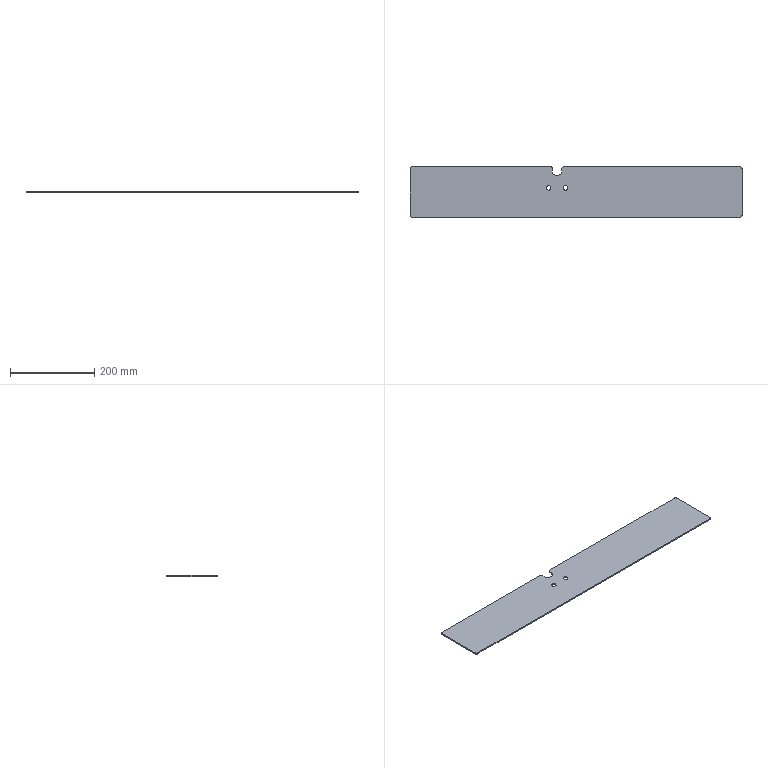Part | STEP file | HL4GD-1.30.103XL cab extended floor plate | 1 solid | 18 faces | box 790 x 120 x 3 mm | volume 282420 mm3 | cylinder 9 | plane 9 | commonest cylinder face diameters 10 x6 11 x2 23 x1
STEP:
#1=CARTESIAN_POINT('',(0.,0.,0.));
#2=DIRECTION('',(0.,0.,1.));
#3=DIRECTION('',(1.,0.,0.));
#4=AXIS2_PLACEMENT_3D('',#1,#2,#3);
#5=CARTESIAN_POINT('',(2036.5,1130.,465.));
#6=VERTEX_POINT('',#5);
#7=CARTESIAN_POINT('',(2013.5,1130.,465.));
#8=VERTEX_POINT('',#7);
#9=CARTESIAN_POINT('',(2025.,1130.,465.));
#10=DIRECTION('',(0.,0.,-1.));
#11=DIRECTION('',(0.,1.,0.));
#12=AXIS2_PLACEMENT_3D('',#9,#10,#11);
#13=CIRCLE('',#12,11.5);
#14=CARTESIAN_POINT('',(2025.,1130.,815.));
#15=DIRECTION('',(0.,0.,-1.));
#16=DIRECTION('',(-1.,0.,0.));
#17=AXIS2_PLACEMENT_3D('',#14,#15,#16);
#18=CYLINDRICAL_SURFACE('',#17,11.5);
#19=CARTESIAN_POINT('',(1.571,350.));
#20=DIRECTION('',(1.,0.));
#21=VECTOR('',#20,1.);
#22=LINE('',#19,#21);
#23=(GEOMETRIC_REPRESENTATION_CONTEXT(2)PARAMETRIC_REPRESENTATION_CONTEXT()REPRESENTATION_CONTEXT('',''));
#24=DEFINITIONAL_REPRESENTATION('',(#22),#23);
#25=PCURVE('',#18,#24);
#26=CARTESIAN_POINT('',(2495.,1140.,465.));
#27=DIRECTION('',(0.,0.,-1.));
#28=DIRECTION('',(0.,1.,0.));
#29=AXIS2_PLACEMENT_3D('',#26,#27,#28);
#30=PLANE('',#29);
#31=CARTESIAN_POINT('',(-10.,-470.));
#32=DIRECTION('',(1.,0.));
#33=AXIS2_PLACEMENT_2D('',#31,#32);
#34=CIRCLE('',#33,11.5);
#35=(GEOMETRIC_REPRESENTATION_CONTEXT(2)PARAMETRIC_REPRESENTATION_CONTEXT()REPRESENTATION_CONTEXT('',''));
#36=DEFINITIONAL_REPRESENTATION('',(#34),#35);
#37=PCURVE('',#30,#36);
#38=SURFACE_CURVE('',#13,(#25,#37),.PCURVE_S1.);
#39=EDGE_CURVE('',#6,#8,#38,.T.);
#40=ORIENTED_EDGE('',*,*,#39,.F.);
#41=CARTESIAN_POINT('',(2036.5,1130.,468.));
#42=VERTEX_POINT('',#41);
#43=CARTESIAN_POINT('',(2036.5,1130.,468.));
#44=DIRECTION('',(0.,0.,1.));
#45=VECTOR('',#44,1.);
#46=LINE('',#43,#45);
#47=CARTESIAN_POINT('',(3.142,347.));
#48=DIRECTION('',(0.,-1.));
#49=VECTOR('',#48,1.);
#50=LINE('',#47,#49);
#51=(GEOMETRIC_REPRESENTATION_CONTEXT(2)PARAMETRIC_REPRESENTATION_CONTEXT()REPRESENTATION_CONTEXT('',''));
#52=DEFINITIONAL_REPRESENTATION('',(#50),#51);
#53=PCURVE('',#18,#52);
#54=CARTESIAN_POINT('',(2036.5,1168.5,468.));
#55=DIRECTION('',(1.,0.,0.));
#56=DIRECTION('',(0.,0.,-1.));
#57=AXIS2_PLACEMENT_3D('',#54,#55,#56);
#58=PLANE('',#57);
#59=CARTESIAN_POINT('',(0.,-38.5));
#60=DIRECTION('',(-1.,0.));
#61=VECTOR('',#60,1.);
#62=LINE('',#59,#61);
#63=(GEOMETRIC_REPRESENTATION_CONTEXT(2)PARAMETRIC_REPRESENTATION_CONTEXT()REPRESENTATION_CONTEXT('',''));
#64=DEFINITIONAL_REPRESENTATION('',(#62),#63);
#65=PCURVE('',#58,#64);
#66=SURFACE_CURVE('',#46,(#53,#65),.PCURVE_S1.);
#67=EDGE_CURVE('',#6,#42,#66,.T.);
#68=ORIENTED_EDGE('',*,*,#67,.T.);
#69=CARTESIAN_POINT('',(2013.5,1130.,468.));
#70=VERTEX_POINT('',#69);
#71=CARTESIAN_POINT('',(2025.,1130.,468.));
#72=DIRECTION('',(0.,0.,-1.));
#73=DIRECTION('',(0.,1.,0.));
#74=AXIS2_PLACEMENT_3D('',#71,#72,#73);
#75=CIRCLE('',#74,11.5);
#76=CARTESIAN_POINT('',(1.571,347.));
#77=DIRECTION('',(1.,0.));
#78=VECTOR('',#77,1.);
#79=LINE('',#76,#78);
#80=(GEOMETRIC_REPRESENTATION_CONTEXT(2)PARAMETRIC_REPRESENTATION_CONTEXT()REPRESENTATION_CONTEXT('',''));
#81=DEFINITIONAL_REPRESENTATION('',(#79),#80);
#82=PCURVE('',#18,#81);
#83=CARTESIAN_POINT('',(2495.,1140.,468.));
#84=DIRECTION('',(0.,0.,-1.));
#85=DIRECTION('',(0.,1.,0.));
#86=AXIS2_PLACEMENT_3D('',#83,#84,#85);
#87=PLANE('',#86);
#88=CARTESIAN_POINT('',(-10.,-470.));
#89=DIRECTION('',(1.,0.));
#90=AXIS2_PLACEMENT_2D('',#88,#89);
#91=CIRCLE('',#90,11.5);
#92=(GEOMETRIC_REPRESENTATION_CONTEXT(2)PARAMETRIC_REPRESENTATION_CONTEXT()REPRESENTATION_CONTEXT('',''));
#93=DEFINITIONAL_REPRESENTATION('',(#91),#92);
#94=PCURVE('',#87,#93);
#95=SURFACE_CURVE('',#75,(#82,#94),.PCURVE_S1.);
#96=EDGE_CURVE('',#42,#70,#95,.T.);
#97=ORIENTED_EDGE('',*,*,#96,.T.);
#98=CARTESIAN_POINT('',(2013.5,1130.,468.));
#99=DIRECTION('',(0.,0.,1.));
#100=VECTOR('',#99,1.);
#101=LINE('',#98,#100);
#102=CARTESIAN_POINT('',(6.283,347.));
#103=DIRECTION('',(0.,-1.));
#104=VECTOR('',#103,1.);
#105=LINE('',#102,#104);
#106=(GEOMETRIC_REPRESENTATION_CONTEXT(2)PARAMETRIC_REPRESENTATION_CONTEXT()REPRESENTATION_CONTEXT('',''));
#107=DEFINITIONAL_REPRESENTATION('',(#105),#106);
#108=PCURVE('',#18,#107);
#109=CARTESIAN_POINT('',(2013.5,1168.5,468.));
#110=DIRECTION('',(-1.,0.,0.));
#111=DIRECTION('',(0.,0.,1.));
#112=AXIS2_PLACEMENT_3D('',#109,#110,#111);
#113=PLANE('',#112);
#114=CARTESIAN_POINT('',(0.,-38.5));
#115=DIRECTION('',(1.,0.));
#116=VECTOR('',#115,1.);
#117=LINE('',#114,#116);
#118=(GEOMETRIC_REPRESENTATION_CONTEXT(2)PARAMETRIC_REPRESENTATION_CONTEXT()REPRESENTATION_CONTEXT('',''));
#119=DEFINITIONAL_REPRESENTATION('',(#117),#118);
#120=PCURVE('',#113,#119);
#121=SURFACE_CURVE('',#101,(#108,#120),.PCURVE_S1.);
#122=EDGE_CURVE('',#8,#70,#121,.T.);
#123=ORIENTED_EDGE('',*,*,#122,.F.);
#124=EDGE_LOOP('',(#40,#68,#97,#123));
#125=FACE_BOUND('',#124,.F.);
#126=ADVANCED_FACE('',(#125),#18,.F.);
#127=CARTESIAN_POINT('',(2041.5,1140.,468.));
#128=VERTEX_POINT('',#127);
#129=CARTESIAN_POINT('',(2460.,1140.,468.));
#130=VERTEX_POINT('',#129);
#131=CARTESIAN_POINT('',(2495.,1140.,468.));
#132=DIRECTION('',(1.,0.,0.));
#133=VECTOR('',#132,1.);
#134=LINE('',#131,#133);
#135=CARTESIAN_POINT('',(2495.,1140.,465.));
#136=DIRECTION('',(0.,1.,0.));
#137=DIRECTION('',(1.,0.,0.));
#138=AXIS2_PLACEMENT_3D('',#135,#136,#137);
#139=PLANE('',#138);
#140=CARTESIAN_POINT('',(0.,-3.));
#141=DIRECTION('',(1.,0.));
#142=VECTOR('',#141,1.);
#143=LINE('',#140,#142);
#144=(GEOMETRIC_REPRESENTATION_CONTEXT(2)PARAMETRIC_REPRESENTATION_CONTEXT()REPRESENTATION_CONTEXT('',''));
#145=DEFINITIONAL_REPRESENTATION('',(#143),#144);
#146=PCURVE('',#139,#145);
#147=CARTESIAN_POINT('',(0.,0.));
#148=DIRECTION('',(0.,1.));
#149=VECTOR('',#148,1.);
#150=LINE('',#147,#149);
#151=(GEOMETRIC_REPRESENTATION_CONTEXT(2)PARAMETRIC_REPRESENTATION_CONTEXT()REPRESENTATION_CONTEXT('',''));
#152=DEFINITIONAL_REPRESENTATION('',(#150),#151);
#153=PCURVE('',#87,#152);
#154=SURFACE_CURVE('',#134,(#146,#153),.PCURVE_S1.);
#155=EDGE_CURVE('',#128,#130,#154,.T.);
#156=ORIENTED_EDGE('',*,*,#155,.T.);
#157=CARTESIAN_POINT('',(2460.,1140.,465.));
#158=VERTEX_POINT('',#157);
#159=CARTESIAN_POINT('',(2460.,1140.,465.));
#160=DIRECTION('',(0.,0.,-1.));
#161=VECTOR('',#160,1.);
#162=LINE('',#159,#161);
#163=CARTESIAN_POINT('',(-35.,0.));
#164=DIRECTION('',(0.,1.));
#165=VECTOR('',#164,1.);
#166=LINE('',#163,#165);
#167=(GEOMETRIC_REPRESENTATION_CONTEXT(2)PARAMETRIC_REPRESENTATION_CONTEXT()REPRESENTATION_CONTEXT('',''));
#168=DEFINITIONAL_REPRESENTATION('',(#166),#167);
#169=PCURVE('',#139,#168);
#170=CARTESIAN_POINT('',(2460.,1135.,465.));
#171=DIRECTION('',(0.,0.,-1.));
#172=DIRECTION('',(0.,1.,0.));
#173=AXIS2_PLACEMENT_3D('',#170,#171,#172);
#174=CYLINDRICAL_SURFACE('',#173,5.);
#175=CARTESIAN_POINT('',(0.,0.));
#176=DIRECTION('',(0.,1.));
#177=VECTOR('',#176,1.);
#178=LINE('',#175,#177);
#179=(GEOMETRIC_REPRESENTATION_CONTEXT(2)PARAMETRIC_REPRESENTATION_CONTEXT()REPRESENTATION_CONTEXT('',''));
#180=DEFINITIONAL_REPRESENTATION('',(#178),#179);
#181=PCURVE('',#174,#180);
#182=SURFACE_CURVE('',#162,(#169,#181),.PCURVE_S1.);
#183=EDGE_CURVE('',#130,#158,#182,.T.);
#184=ORIENTED_EDGE('',*,*,#183,.T.);
#185=CARTESIAN_POINT('',(2041.5,1140.,465.));
#186=VERTEX_POINT('',#185);
#187=CARTESIAN_POINT('',(2495.,1140.,465.));
#188=DIRECTION('',(1.,0.,0.));
#189=VECTOR('',#188,1.);
#190=LINE('',#187,#189);
#191=CARTESIAN_POINT('',(0.,0.));
#192=DIRECTION('',(1.,0.));
#193=VECTOR('',#192,1.);
#194=LINE('',#191,#193);
#195=(GEOMETRIC_REPRESENTATION_CONTEXT(2)PARAMETRIC_REPRESENTATION_CONTEXT()REPRESENTATION_CONTEXT('',''));
#196=DEFINITIONAL_REPRESENTATION('',(#194),#195);
#197=PCURVE('',#139,#196);
#198=CARTESIAN_POINT('',(0.,0.));
#199=DIRECTION('',(0.,1.));
#200=VECTOR('',#199,1.);
#201=LINE('',#198,#200);
#202=(GEOMETRIC_REPRESENTATION_CONTEXT(2)PARAMETRIC_REPRESENTATION_CONTEXT()REPRESENTATION_CONTEXT('',''));
#203=DEFINITIONAL_REPRESENTATION('',(#201),#202);
#204=PCURVE('',#30,#203);
#205=SURFACE_CURVE('',#190,(#197,#204),.PCURVE_S1.);
#206=EDGE_CURVE('',#186,#158,#205,.T.);
#207=ORIENTED_EDGE('',*,*,#206,.F.);
#208=CARTESIAN_POINT('',(2041.5,1140.,468.));
#209=DIRECTION('',(0.,0.,1.));
#210=VECTOR('',#209,1.);
#211=LINE('',#208,#210);
#212=CARTESIAN_POINT('',(-453.5,-3.));
#213=DIRECTION('',(0.,-1.));
#214=VECTOR('',#213,1.);
#215=LINE('',#212,#214);
#216=(GEOMETRIC_REPRESENTATION_CONTEXT(2)PARAMETRIC_REPRESENTATION_CONTEXT()REPRESENTATION_CONTEXT('',''));
#217=DEFINITIONAL_REPRESENTATION('',(#215),#216);
#218=PCURVE('',#139,#217);
#219=CARTESIAN_POINT('',(2041.5,1135.,468.));
#220=DIRECTION('',(0.,0.,1.));
#221=DIRECTION('',(0.,-1.,0.));
#222=AXIS2_PLACEMENT_3D('',#219,#220,#221);
#223=CYLINDRICAL_SURFACE('',#222,5.);
#224=CARTESIAN_POINT('',(3.142,0.));
#225=DIRECTION('',(0.,1.));
#226=VECTOR('',#225,1.);
#227=LINE('',#224,#226);
#228=(GEOMETRIC_REPRESENTATION_CONTEXT(2)PARAMETRIC_REPRESENTATION_CONTEXT()REPRESENTATION_CONTEXT('',''));
#229=DEFINITIONAL_REPRESENTATION('',(#227),#228);
#230=PCURVE('',#223,#229);
#231=SURFACE_CURVE('',#211,(#218,#230),.PCURVE_S1.);
#232=EDGE_CURVE('',#186,#128,#231,.T.);
#233=ORIENTED_EDGE('',*,*,#232,.T.);
#234=EDGE_LOOP('',(#156,#184,#207,#233));
#235=FACE_BOUND('',#234,.T.);
#236=ADVANCED_FACE('',(#235),#139,.T.);
#237=CARTESIAN_POINT('',(1680.,1140.,465.));
#238=VERTEX_POINT('',#237);
#239=CARTESIAN_POINT('',(2008.5,1140.,465.));
#240=VERTEX_POINT('',#239);
#241=CARTESIAN_POINT('',(2495.,1140.,465.));
#242=DIRECTION('',(1.,0.,0.));
#243=VECTOR('',#242,1.);
#244=LINE('',#241,#243);
#245=CARTESIAN_POINT('',(2495.,1140.,465.));
#246=DIRECTION('',(0.,1.,0.));
#247=DIRECTION('',(1.,0.,0.));
#248=AXIS2_PLACEMENT_3D('',#245,#246,#247);
#249=PLANE('',#248);
#250=CARTESIAN_POINT('',(0.,0.));
#251=DIRECTION('',(1.,0.));
#252=VECTOR('',#251,1.);
#253=LINE('',#250,#252);
#254=(GEOMETRIC_REPRESENTATION_CONTEXT(2)PARAMETRIC_REPRESENTATION_CONTEXT()REPRESENTATION_CONTEXT('',''));
#255=DEFINITIONAL_REPRESENTATION('',(#253),#254);
#256=PCURVE('',#249,#255);
#257=CARTESIAN_POINT('',(0.,0.));
#258=DIRECTION('',(0.,1.));
#259=VECTOR('',#258,1.);
#260=LINE('',#257,#259);
#261=(GEOMETRIC_REPRESENTATION_CONTEXT(2)PARAMETRIC_REPRESENTATION_CONTEXT()REPRESENTATION_CONTEXT('',''));
#262=DEFINITIONAL_REPRESENTATION('',(#260),#261);
#263=PCURVE('',#30,#262);
#264=SURFACE_CURVE('',#244,(#256,#263),.PCURVE_S1.);
#265=EDGE_CURVE('',#238,#240,#264,.T.);
#266=ORIENTED_EDGE('',*,*,#265,.F.);
#267=CARTESIAN_POINT('',(1680.,1140.,468.));
#268=VERTEX_POINT('',#267);
#269=CARTESIAN_POINT('',(1680.,1140.,465.));
#270=DIRECTION('',(0.,0.,1.));
#271=VECTOR('',#270,1.);
#272=LINE('',#269,#271);
#273=CARTESIAN_POINT('',(-815.,0.));
#274=DIRECTION('',(0.,-1.));
#275=VECTOR('',#274,1.);
#276=LINE('',#273,#275);
#277=(GEOMETRIC_REPRESENTATION_CONTEXT(2)PARAMETRIC_REPRESENTATION_CONTEXT()REPRESENTATION_CONTEXT('',''));
#278=DEFINITIONAL_REPRESENTATION('',(#276),#277);
#279=PCURVE('',#249,#278);
#280=CARTESIAN_POINT('',(1680.,1135.,465.));
#281=DIRECTION('',(0.,0.,1.));
#282=DIRECTION('',(0.,-1.,0.));
#283=AXIS2_PLACEMENT_3D('',#280,#281,#282);
#284=CYLINDRICAL_SURFACE('',#283,5.);
#285=CARTESIAN_POINT('',(3.142,0.));
#286=DIRECTION('',(0.,1.));
#287=VECTOR('',#286,1.);
#288=LINE('',#285,#287);
#289=(GEOMETRIC_REPRESENTATION_CONTEXT(2)PARAMETRIC_REPRESENTATION_CONTEXT()REPRESENTATION_CONTEXT('',''));
#290=DEFINITIONAL_REPRESENTATION('',(#288),#289);
#291=PCURVE('',#284,#290);
#292=SURFACE_CURVE('',#272,(#279,#291),.PCURVE_S1.);
#293=EDGE_CURVE('',#238,#268,#292,.T.);
#294=ORIENTED_EDGE('',*,*,#293,.T.);
#295=CARTESIAN_POINT('',(2008.5,1140.,468.));
#296=VERTEX_POINT('',#295);
#297=CARTESIAN_POINT('',(2495.,1140.,468.));
#298=DIRECTION('',(1.,0.,0.));
#299=VECTOR('',#298,1.);
#300=LINE('',#297,#299);
#301=CARTESIAN_POINT('',(0.,-3.));
#302=DIRECTION('',(1.,0.));
#303=VECTOR('',#302,1.);
#304=LINE('',#301,#303);
#305=(GEOMETRIC_REPRESENTATION_CONTEXT(2)PARAMETRIC_REPRESENTATION_CONTEXT()REPRESENTATION_CONTEXT('',''));
#306=DEFINITIONAL_REPRESENTATION('',(#304),#305);
#307=PCURVE('',#249,#306);
#308=CARTESIAN_POINT('',(0.,0.));
#309=DIRECTION('',(0.,1.));
#310=VECTOR('',#309,1.);
#311=LINE('',#308,#310);
#312=(GEOMETRIC_REPRESENTATION_CONTEXT(2)PARAMETRIC_REPRESENTATION_CONTEXT()REPRESENTATION_CONTEXT('',''));
#313=DEFINITIONAL_REPRESENTATION('',(#311),#312);
#314=PCURVE('',#87,#313);
#315=SURFACE_CURVE('',#300,(#307,#314),.PCURVE_S1.);
#316=EDGE_CURVE('',#268,#296,#315,.T.);
#317=ORIENTED_EDGE('',*,*,#316,.T.);
#318=CARTESIAN_POINT('',(2008.5,1140.,465.));
#319=DIRECTION('',(0.,0.,-1.));
#320=VECTOR('',#319,1.);
#321=LINE('',#318,#320);
#322=CARTESIAN_POINT('',(-486.5,0.));
#323=DIRECTION('',(0.,1.));
#324=VECTOR('',#323,1.);
#325=LINE('',#322,#324);
#326=(GEOMETRIC_REPRESENTATION_CONTEXT(2)PARAMETRIC_REPRESENTATION_CONTEXT()REPRESENTATION_CONTEXT('',''));
#327=DEFINITIONAL_REPRESENTATION('',(#325),#326);
#328=PCURVE('',#249,#327);
#329=CARTESIAN_POINT('',(2008.5,1135.,468.));
#330=DIRECTION('',(0.,0.,-1.));
#331=DIRECTION('',(0.,1.,0.));
#332=AXIS2_PLACEMENT_3D('',#329,#330,#331);
#333=CYLINDRICAL_SURFACE('',#332,5.);
#334=CARTESIAN_POINT('',(0.,3.));
#335=DIRECTION('',(0.,1.));
#336=VECTOR('',#335,1.);
#337=LINE('',#334,#336);
#338=(GEOMETRIC_REPRESENTATION_CONTEXT(2)PARAMETRIC_REPRESENTATION_CONTEXT()REPRESENTATION_CONTEXT('',''));
#339=DEFINITIONAL_REPRESENTATION('',(#337),#338);
#340=PCURVE('',#333,#339);
#341=SURFACE_CURVE('',#321,(#328,#340),.PCURVE_S1.);
#342=EDGE_CURVE('',#296,#240,#341,.T.);
#343=ORIENTED_EDGE('',*,*,#342,.T.);
#344=EDGE_LOOP('',(#266,#294,#317,#343));
#345=FACE_BOUND('',#344,.T.);
#346=ADVANCED_FACE('',(#345),#249,.T.);
#347=CARTESIAN_POINT('',(1680.,1020.,468.));
#348=VERTEX_POINT('',#347);
#349=CARTESIAN_POINT('',(2460.,1020.,468.));
#350=VERTEX_POINT('',#349);
#351=CARTESIAN_POINT('',(2495.,1020.,468.));
#352=DIRECTION('',(1.,0.,0.));
#353=VECTOR('',#352,1.);
#354=LINE('',#351,#353);
#355=CARTESIAN_POINT('',(2495.,1020.,465.));
#356=DIRECTION('',(0.,1.,0.));
#357=DIRECTION('',(1.,0.,0.));
#358=AXIS2_PLACEMENT_3D('',#355,#356,#357);
#359=PLANE('',#358);
#360=CARTESIAN_POINT('',(0.,-3.));
#361=DIRECTION('',(1.,0.));
#362=VECTOR('',#361,1.);
#363=LINE('',#360,#362);
#364=(GEOMETRIC_REPRESENTATION_CONTEXT(2)PARAMETRIC_REPRESENTATION_CONTEXT()REPRESENTATION_CONTEXT('',''));
#365=DEFINITIONAL_REPRESENTATION('',(#363),#364);
#366=PCURVE('',#359,#365);
#367=CARTESIAN_POINT('',(-120.,0.));
#368=DIRECTION('',(0.,1.));
#369=VECTOR('',#368,1.);
#370=LINE('',#367,#369);
#371=(GEOMETRIC_REPRESENTATION_CONTEXT(2)PARAMETRIC_REPRESENTATION_CONTEXT()REPRESENTATION_CONTEXT('',''));
#372=DEFINITIONAL_REPRESENTATION('',(#370),#371);
#373=PCURVE('',#87,#372);
#374=SURFACE_CURVE('',#354,(#366,#373),.PCURVE_S1.);
#375=EDGE_CURVE('',#348,#350,#374,.T.);
#376=ORIENTED_EDGE('',*,*,#375,.F.);
#377=CARTESIAN_POINT('',(1680.,1020.,465.));
#378=VERTEX_POINT('',#377);
#379=CARTESIAN_POINT('',(1680.,1020.,465.));
#380=DIRECTION('',(0.,0.,-1.));
#381=VECTOR('',#380,1.);
#382=LINE('',#379,#381);
#383=CARTESIAN_POINT('',(-815.,0.));
#384=DIRECTION('',(0.,1.));
#385=VECTOR('',#384,1.);
#386=LINE('',#383,#385);
#387=(GEOMETRIC_REPRESENTATION_CONTEXT(2)PARAMETRIC_REPRESENTATION_CONTEXT()REPRESENTATION_CONTEXT('',''));
#388=DEFINITIONAL_REPRESENTATION('',(#386),#387);
#389=PCURVE('',#359,#388);
#390=CARTESIAN_POINT('',(1680.,1025.,465.));
#391=DIRECTION('',(0.,0.,1.));
#392=DIRECTION('',(0.,-1.,0.));
#393=AXIS2_PLACEMENT_3D('',#390,#391,#392);
#394=CYLINDRICAL_SURFACE('',#393,5.);
#395=CARTESIAN_POINT('',(6.283,0.));
#396=DIRECTION('',(0.,-1.));
#397=VECTOR('',#396,1.);
#398=LINE('',#395,#397);
#399=(GEOMETRIC_REPRESENTATION_CONTEXT(2)PARAMETRIC_REPRESENTATION_CONTEXT()REPRESENTATION_CONTEXT('',''));
#400=DEFINITIONAL_REPRESENTATION('',(#398),#399);
#401=PCURVE('',#394,#400);
#402=SURFACE_CURVE('',#382,(#389,#401),.PCURVE_S1.);
#403=EDGE_CURVE('',#348,#378,#402,.T.);
#404=ORIENTED_EDGE('',*,*,#403,.T.);
#405=CARTESIAN_POINT('',(2460.,1020.,465.));
#406=VERTEX_POINT('',#405);
#407=CARTESIAN_POINT('',(2495.,1020.,465.));
#408=DIRECTION('',(1.,0.,0.));
#409=VECTOR('',#408,1.);
#410=LINE('',#407,#409);
#411=CARTESIAN_POINT('',(0.,0.));
#412=DIRECTION('',(1.,0.));
#413=VECTOR('',#412,1.);
#414=LINE('',#411,#413);
#415=(GEOMETRIC_REPRESENTATION_CONTEXT(2)PARAMETRIC_REPRESENTATION_CONTEXT()REPRESENTATION_CONTEXT('',''));
#416=DEFINITIONAL_REPRESENTATION('',(#414),#415);
#417=PCURVE('',#359,#416);
#418=CARTESIAN_POINT('',(-120.,0.));
#419=DIRECTION('',(0.,1.));
#420=VECTOR('',#419,1.);
#421=LINE('',#418,#420);
#422=(GEOMETRIC_REPRESENTATION_CONTEXT(2)PARAMETRIC_REPRESENTATION_CONTEXT()REPRESENTATION_CONTEXT('',''));
#423=DEFINITIONAL_REPRESENTATION('',(#421),#422);
#424=PCURVE('',#30,#423);
#425=SURFACE_CURVE('',#410,(#417,#424),.PCURVE_S1.);
#426=EDGE_CURVE('',#378,#406,#425,.T.);
#427=ORIENTED_EDGE('',*,*,#426,.T.);
#428=CARTESIAN_POINT('',(2460.,1020.,465.));
#429=DIRECTION('',(0.,0.,1.));
#430=VECTOR('',#429,1.);
#431=LINE('',#428,#430);
#432=CARTESIAN_POINT('',(-35.,0.));
#433=DIRECTION('',(0.,-1.));
#434=VECTOR('',#433,1.);
#435=LINE('',#432,#434);
#436=(GEOMETRIC_REPRESENTATION_CONTEXT(2)PARAMETRIC_REPRESENTATION_CONTEXT()REPRESENTATION_CONTEXT('',''));
#437=DEFINITIONAL_REPRESENTATION('',(#435),#436);
#438=PCURVE('',#359,#437);
#439=CARTESIAN_POINT('',(2460.,1025.,465.));
#440=DIRECTION('',(0.,0.,-1.));
#441=DIRECTION('',(0.,1.,0.));
#442=AXIS2_PLACEMENT_3D('',#439,#440,#441);
#443=CYLINDRICAL_SURFACE('',#442,5.);
#444=CARTESIAN_POINT('',(3.142,0.));
#445=DIRECTION('',(0.,-1.));
#446=VECTOR('',#445,1.);
#447=LINE('',#444,#446);
#448=(GEOMETRIC_REPRESENTATION_CONTEXT(2)PARAMETRIC_REPRESENTATION_CONTEXT()REPRESENTATION_CONTEXT('',''));
#449=DEFINITIONAL_REPRESENTATION('',(#447),#448);
#450=PCURVE('',#443,#449);
#451=SURFACE_CURVE('',#431,(#438,#450),.PCURVE_S1.);
#452=EDGE_CURVE('',#406,#350,#451,.T.);
#453=ORIENTED_EDGE('',*,*,#452,.T.);
#454=EDGE_LOOP('',(#376,#404,#427,#453));
#455=FACE_BOUND('',#454,.T.);
#456=ADVANCED_FACE('',(#455),#359,.F.);
#457=CARTESIAN_POINT('',(2045.,1095.5,468.));
#458=VERTEX_POINT('',#457);
#459=CARTESIAN_POINT('',(2045.,1090.,468.));
#460=DIRECTION('',(0.,0.,1.));
#461=DIRECTION('',(0.,1.,0.));
#462=AXIS2_PLACEMENT_3D('',#459,#460,#461);
#463=CIRCLE('',#462,5.5);
#464=CARTESIAN_POINT('',(-44.5,-450.));
#465=CARTESIAN_POINT('',(-44.5,-459.526));
#466=CARTESIAN_POINT('',(-52.75,-454.763));
#467=CARTESIAN_POINT('',(-61.,-450.));
#468=CARTESIAN_POINT('',(-52.75,-445.237));
#469=CARTESIAN_POINT('',(-44.5,-440.474));
#470=CARTESIAN_POINT('',(-44.5,-450.));
#471=(BOUNDED_CURVE()B_SPLINE_CURVE(2,(#464,#465,#466,#467,#468,#469,#470),.UNSPECIFIED.,.T.,.F.)B_SPLINE_CURVE_WITH_KNOTS((1,2,2,2,2,1),(-2.094,0.,2.094,4.189,6.283,8.378),.UNSPECIFIED.)CURVE()GEOMETRIC_REPRESENTATION_ITEM()RATIONAL_B_SPLINE_CURVE((1.,0.5,1.,0.5,1.,0.5,1.))REPRESENTATION_ITEM(''));
#472=(GEOMETRIC_REPRESENTATION_CONTEXT(2)PARAMETRIC_REPRESENTATION_CONTEXT()REPRESENTATION_CONTEXT('',''));
#473=DEFINITIONAL_REPRESENTATION('',(#471),#472);
#474=PCURVE('',#87,#473);
#475=CARTESIAN_POINT('',(2045.,1090.,1419.));
#476=DIRECTION('',(0.,0.,-1.));
#477=DIRECTION('',(-1.,0.,0.));
#478=AXIS2_PLACEMENT_3D('',#475,#476,#477);
#479=CYLINDRICAL_SURFACE('',#478,5.5);
#480=CARTESIAN_POINT('',(7.854,951.));
#481=DIRECTION('',(-1.,0.));
#482=VECTOR('',#481,1.);
#483=LINE('',#480,#482);
#484=(GEOMETRIC_REPRESENTATION_CONTEXT(2)PARAMETRIC_REPRESENTATION_CONTEXT()REPRESENTATION_CONTEXT('',''));
#485=DEFINITIONAL_REPRESENTATION('',(#483),#484);
#486=PCURVE('',#479,#485);
#487=SURFACE_CURVE('',#463,(#474,#486),.PCURVE_S1.);
#488=EDGE_CURVE('',#458,#458,#487,.T.);
#489=ORIENTED_EDGE('',*,*,#488,.F.);
#490=EDGE_LOOP('',(#489));
#491=FACE_BOUND('',#490,.T.);
#492=CARTESIAN_POINT('',(2005.,1095.5,468.));
#493=VERTEX_POINT('',#492);
#494=CARTESIAN_POINT('',(2005.,1090.,468.));
#495=DIRECTION('',(0.,0.,1.));
#496=DIRECTION('',(0.,1.,0.));
#497=AXIS2_PLACEMENT_3D('',#494,#495,#496);
#498=CIRCLE('',#497,5.5);
#499=CARTESIAN_POINT('',(-44.5,-490.));
#500=CARTESIAN_POINT('',(-44.5,-499.526));
#501=CARTESIAN_POINT('',(-52.75,-494.763));
#502=CARTESIAN_POINT('',(-61.,-490.));
#503=CARTESIAN_POINT('',(-52.75,-485.237));
#504=CARTESIAN_POINT('',(-44.5,-480.474));
#505=CARTESIAN_POINT('',(-44.5,-490.));
#506=(BOUNDED_CURVE()B_SPLINE_CURVE(2,(#499,#500,#501,#502,#503,#504,#505),.UNSPECIFIED.,.T.,.F.)B_SPLINE_CURVE_WITH_KNOTS((1,2,2,2,2,1),(-2.094,0.,2.094,4.189,6.283,8.378),.UNSPECIFIED.)CURVE()GEOMETRIC_REPRESENTATION_ITEM()RATIONAL_B_SPLINE_CURVE((1.,0.5,1.,0.5,1.,0.5,1.))REPRESENTATION_ITEM(''));
#507=(GEOMETRIC_REPRESENTATION_CONTEXT(2)PARAMETRIC_REPRESENTATION_CONTEXT()REPRESENTATION_CONTEXT('',''));
#508=DEFINITIONAL_REPRESENTATION('',(#506),#507);
#509=PCURVE('',#87,#508);
#510=CARTESIAN_POINT('',(2005.,1090.,1419.));
#511=DIRECTION('',(0.,0.,-1.));
#512=DIRECTION('',(-1.,0.,0.));
#513=AXIS2_PLACEMENT_3D('',#510,#511,#512);
#514=CYLINDRICAL_SURFACE('',#513,5.5);
#515=CARTESIAN_POINT('',(7.854,951.));
#516=DIRECTION('',(-1.,0.));
#517=VECTOR('',#516,1.);
#518=LINE('',#515,#517);
#519=(GEOMETRIC_REPRESENTATION_CONTEXT(2)PARAMETRIC_REPRESENTATION_CONTEXT()REPRESENTATION_CONTEXT('',''));
#520=DEFINITIONAL_REPRESENTATION('',(#518),#519);
#521=PCURVE('',#514,#520);
#522=SURFACE_CURVE('',#498,(#509,#521),.PCURVE_S1.);
#523=EDGE_CURVE('',#493,#493,#522,.T.);
#524=ORIENTED_EDGE('',*,*,#523,.F.);
#525=EDGE_LOOP('',(#524));
#526=FACE_BOUND('',#525,.T.);
#527=CARTESIAN_POINT('',(1675.,1135.,468.));
#528=VERTEX_POINT('',#527);
#529=CARTESIAN_POINT('',(1675.,1025.,468.));
#530=VERTEX_POINT('',#529);
#531=CARTESIAN_POINT('',(1675.,1140.,468.));
#532=DIRECTION('',(0.,-1.,0.));
#533=VECTOR('',#532,1.);
#534=LINE('',#531,#533);
#535=CARTESIAN_POINT('',(0.,-820.));
#536=DIRECTION('',(-1.,0.));
#537=VECTOR('',#536,1.);
#538=LINE('',#535,#537);
#539=(GEOMETRIC_REPRESENTATION_CONTEXT(2)PARAMETRIC_REPRESENTATION_CONTEXT()REPRESENTATION_CONTEXT('',''));
#540=DEFINITIONAL_REPRESENTATION('',(#538),#539);
#541=PCURVE('',#87,#540);
#542=CARTESIAN_POINT('',(1675.,740.,435.));
#543=DIRECTION('',(-1.,0.,0.));
#544=DIRECTION('',(0.,0.,1.));
#545=AXIS2_PLACEMENT_3D('',#542,#543,#544);
#546=PLANE('',#545);
#547=CARTESIAN_POINT('',(33.,400.));
#548=DIRECTION('',(0.,-1.));
#549=VECTOR('',#548,1.);
#550=LINE('',#547,#549);
#551=(GEOMETRIC_REPRESENTATION_CONTEXT(2)PARAMETRIC_REPRESENTATION_CONTEXT()REPRESENTATION_CONTEXT('',''));
#552=DEFINITIONAL_REPRESENTATION('',(#550),#551);
#553=PCURVE('',#546,#552);
#554=SURFACE_CURVE('',#534,(#541,#553),.PCURVE_S1.);
#555=EDGE_CURVE('',#528,#530,#554,.T.);
#556=ORIENTED_EDGE('',*,*,#555,.T.);
#557=CARTESIAN_POINT('',(1680.,1025.,468.));
#558=DIRECTION('',(0.,0.,1.));
#559=DIRECTION('',(0.,1.,0.));
#560=AXIS2_PLACEMENT_3D('',#557,#558,#559);
#561=CIRCLE('',#560,5.);
#562=CARTESIAN_POINT('',(-110.,-815.));
#563=CARTESIAN_POINT('',(-110.,-823.66));
#564=CARTESIAN_POINT('',(-117.5,-819.33));
#565=CARTESIAN_POINT('',(-125.,-815.));
#566=CARTESIAN_POINT('',(-117.5,-810.67));
#567=CARTESIAN_POINT('',(-110.,-806.34));
#568=CARTESIAN_POINT('',(-110.,-815.));
#569=(BOUNDED_CURVE()B_SPLINE_CURVE(2,(#562,#563,#564,#565,#566,#567,#568),.UNSPECIFIED.,.T.,.F.)B_SPLINE_CURVE_WITH_KNOTS((1,2,2,2,2,1),(-2.094,0.,2.094,4.189,6.283,8.378),.UNSPECIFIED.)CURVE()GEOMETRIC_REPRESENTATION_ITEM()RATIONAL_B_SPLINE_CURVE((1.,0.5,1.,0.5,1.,0.5,1.))REPRESENTATION_ITEM(''));
#570=(GEOMETRIC_REPRESENTATION_CONTEXT(2)PARAMETRIC_REPRESENTATION_CONTEXT()REPRESENTATION_CONTEXT('',''));
#571=DEFINITIONAL_REPRESENTATION('',(#569),#570);
#572=PCURVE('',#87,#571);
#573=CARTESIAN_POINT('',(3.142,3.));
#574=DIRECTION('',(1.,0.));
#575=VECTOR('',#574,1.);
#576=LINE('',#573,#575);
#577=(GEOMETRIC_REPRESENTATION_CONTEXT(2)PARAMETRIC_REPRESENTATION_CONTEXT()REPRESENTATION_CONTEXT('',''));
#578=DEFINITIONAL_REPRESENTATION('',(#576),#577);
#579=PCURVE('',#394,#578);
#580=SURFACE_CURVE('',#561,(#572,#579),.PCURVE_S1.);
#581=EDGE_CURVE('',#530,#348,#580,.T.);
#582=ORIENTED_EDGE('',*,*,#581,.T.);
#583=ORIENTED_EDGE('',*,*,#375,.T.);
#584=CARTESIAN_POINT('',(2465.,1025.,468.));
#585=VERTEX_POINT('',#584);
#586=CARTESIAN_POINT('',(2460.,1025.,468.));
#587=DIRECTION('',(0.,0.,1.));
#588=DIRECTION('',(0.,1.,0.));
#589=AXIS2_PLACEMENT_3D('',#586,#587,#588);
#590=CIRCLE('',#589,5.);
#591=CARTESIAN_POINT('',(-110.,-35.));
#592=CARTESIAN_POINT('',(-110.,-43.66));
#593=CARTESIAN_POINT('',(-117.5,-39.33));
#594=CARTESIAN_POINT('',(-125.,-35.));
#595=CARTESIAN_POINT('',(-117.5,-30.67));
#596=CARTESIAN_POINT('',(-110.,-26.34));
#597=CARTESIAN_POINT('',(-110.,-35.));
#598=(BOUNDED_CURVE()B_SPLINE_CURVE(2,(#591,#592,#593,#594,#595,#596,#597),.UNSPECIFIED.,.T.,.F.)B_SPLINE_CURVE_WITH_KNOTS((1,2,2,2,2,1),(-2.094,0.,2.094,4.189,6.283,8.378),.UNSPECIFIED.)CURVE()GEOMETRIC_REPRESENTATION_ITEM()RATIONAL_B_SPLINE_CURVE((1.,0.5,1.,0.5,1.,0.5,1.))REPRESENTATION_ITEM(''));
#599=(GEOMETRIC_REPRESENTATION_CONTEXT(2)PARAMETRIC_REPRESENTATION_CONTEXT()REPRESENTATION_CONTEXT('',''));
#600=DEFINITIONAL_REPRESENTATION('',(#598),#599);
#601=PCURVE('',#87,#600);
#602=CARTESIAN_POINT('',(6.283,-3.));
#603=DIRECTION('',(-1.,0.));
#604=VECTOR('',#603,1.);
#605=LINE('',#602,#604);
#606=(GEOMETRIC_REPRESENTATION_CONTEXT(2)PARAMETRIC_REPRESENTATION_CONTEXT()REPRESENTATION_CONTEXT('',''));
#607=DEFINITIONAL_REPRESENTATION('',(#605),#606);
#608=PCURVE('',#443,#607);
#609=SURFACE_CURVE('',#590,(#601,#608),.PCURVE_S1.);
#610=EDGE_CURVE('',#350,#585,#609,.T.);
#611=ORIENTED_EDGE('',*,*,#610,.T.);
#612=CARTESIAN_POINT('',(2465.,1135.,468.));
#613=VERTEX_POINT('',#612);
#614=CARTESIAN_POINT('',(2465.,1140.,468.));
#615=DIRECTION('',(0.,1.,0.));
#616=VECTOR('',#615,1.);
#617=LINE('',#614,#616);
#618=CARTESIAN_POINT('',(0.,-30.));
#619=DIRECTION('',(1.,0.));
#620=VECTOR('',#619,1.);
#621=LINE('',#618,#620);
#622=(GEOMETRIC_REPRESENTATION_CONTEXT(2)PARAMETRIC_REPRESENTATION_CONTEXT()REPRESENTATION_CONTEXT('',''));
#623=DEFINITIONAL_REPRESENTATION('',(#621),#622);
#624=PCURVE('',#87,#623);
#625=CARTESIAN_POINT('',(2465.,820.,435.));
#626=DIRECTION('',(1.,0.,0.));
#627=DIRECTION('',(0.,0.,-1.));
#628=AXIS2_PLACEMENT_3D('',#625,#626,#627);
#629=PLANE('',#628);
#630=CARTESIAN_POINT('',(-33.,320.));
#631=DIRECTION('',(0.,1.));
#632=VECTOR('',#631,1.);
#633=LINE('',#630,#632);
#634=(GEOMETRIC_REPRESENTATION_CONTEXT(2)PARAMETRIC_REPRESENTATION_CONTEXT()REPRESENTATION_CONTEXT('',''));
#635=DEFINITIONAL_REPRESENTATION('',(#633),#634);
#636=PCURVE('',#629,#635);
#637=SURFACE_CURVE('',#617,(#624,#636),.PCURVE_S1.);
#638=EDGE_CURVE('',#585,#613,#637,.T.);
#639=ORIENTED_EDGE('',*,*,#638,.T.);
#640=CARTESIAN_POINT('',(2460.,1135.,468.));
#641=DIRECTION('',(0.,0.,1.));
#642=DIRECTION('',(0.,1.,0.));
#643=AXIS2_PLACEMENT_3D('',#640,#641,#642);
#644=CIRCLE('',#643,5.);
#645=CARTESIAN_POINT('',(0.,-35.));
#646=CARTESIAN_POINT('',(0.,-43.66));
#647=CARTESIAN_POINT('',(-7.5,-39.33));
#648=CARTESIAN_POINT('',(-15.,-35.));
#649=CARTESIAN_POINT('',(-7.5,-30.67));
#650=CARTESIAN_POINT('',(0.,-26.34));
#651=CARTESIAN_POINT('',(0.,-35.));
#652=(BOUNDED_CURVE()B_SPLINE_CURVE(2,(#645,#646,#647,#648,#649,#650,#651),.UNSPECIFIED.,.T.,.F.)B_SPLINE_CURVE_WITH_KNOTS((1,2,2,2,2,1),(-2.094,0.,2.094,4.189,6.283,8.378),.UNSPECIFIED.)CURVE()GEOMETRIC_REPRESENTATION_ITEM()RATIONAL_B_SPLINE_CURVE((1.,0.5,1.,0.5,1.,0.5,1.))REPRESENTATION_ITEM(''));
#653=(GEOMETRIC_REPRESENTATION_CONTEXT(2)PARAMETRIC_REPRESENTATION_CONTEXT()REPRESENTATION_CONTEXT('',''));
#654=DEFINITIONAL_REPRESENTATION('',(#652),#653);
#655=PCURVE('',#87,#654);
#656=CARTESIAN_POINT('',(6.283,-3.));
#657=DIRECTION('',(-1.,0.));
#658=VECTOR('',#657,1.);
#659=LINE('',#656,#658);
#660=(GEOMETRIC_REPRESENTATION_CONTEXT(2)PARAMETRIC_REPRESENTATION_CONTEXT()REPRESENTATION_CONTEXT('',''));
#661=DEFINITIONAL_REPRESENTATION('',(#659),#660);
#662=PCURVE('',#174,#661);
#663=SURFACE_CURVE('',#644,(#655,#662),.PCURVE_S1.);
#664=EDGE_CURVE('',#613,#130,#663,.T.);
#665=ORIENTED_EDGE('',*,*,#664,.T.);
#666=ORIENTED_EDGE('',*,*,#155,.F.);
#667=CARTESIAN_POINT('',(2036.5,1135.,468.));
#668=VERTEX_POINT('',#667);
#669=CARTESIAN_POINT('',(2041.5,1135.,468.));
#670=DIRECTION('',(0.,0.,1.));
#671=DIRECTION('',(0.,1.,0.));
#672=AXIS2_PLACEMENT_3D('',#669,#670,#671);
#673=CIRCLE('',#672,5.);
#674=CARTESIAN_POINT('',(0.,-453.5));
#675=CARTESIAN_POINT('',(0.,-462.16));
#676=CARTESIAN_POINT('',(-7.5,-457.83));
#677=CARTESIAN_POINT('',(-15.,-453.5));
#678=CARTESIAN_POINT('',(-7.5,-449.17));
#679=CARTESIAN_POINT('',(0.,-444.84));
#680=CARTESIAN_POINT('',(0.,-453.5));
#681=(BOUNDED_CURVE()B_SPLINE_CURVE(2,(#674,#675,#676,#677,#678,#679,#680),.UNSPECIFIED.,.T.,.F.)B_SPLINE_CURVE_WITH_KNOTS((1,2,2,2,2,1),(-2.094,0.,2.094,4.189,6.283,8.378),.UNSPECIFIED.)CURVE()GEOMETRIC_REPRESENTATION_ITEM()RATIONAL_B_SPLINE_CURVE((1.,0.5,1.,0.5,1.,0.5,1.))REPRESENTATION_ITEM(''));
#682=(GEOMETRIC_REPRESENTATION_CONTEXT(2)PARAMETRIC_REPRESENTATION_CONTEXT()REPRESENTATION_CONTEXT('',''));
#683=DEFINITIONAL_REPRESENTATION('',(#681),#682);
#684=PCURVE('',#87,#683);
#685=CARTESIAN_POINT('',(3.142,0.));
#686=DIRECTION('',(1.,0.));
#687=VECTOR('',#686,1.);
#688=LINE('',#685,#687);
#689=(GEOMETRIC_REPRESENTATION_CONTEXT(2)PARAMETRIC_REPRESENTATION_CONTEXT()REPRESENTATION_CONTEXT('',''));
#690=DEFINITIONAL_REPRESENTATION('',(#688),#689);
#691=PCURVE('',#223,#690);
#692=SURFACE_CURVE('',#673,(#684,#691),.PCURVE_S1.);
#693=EDGE_CURVE('',#128,#668,#692,.T.);
#694=ORIENTED_EDGE('',*,*,#693,.T.);
#695=CARTESIAN_POINT('',(2036.5,1168.5,468.));
#696=DIRECTION('',(0.,1.,0.));
#697=VECTOR('',#696,1.);
#698=LINE('',#695,#697);
#699=CARTESIAN_POINT('',(28.5,-458.5));
#700=DIRECTION('',(1.,0.));
#701=VECTOR('',#700,1.);
#702=LINE('',#699,#701);
#703=(GEOMETRIC_REPRESENTATION_CONTEXT(2)PARAMETRIC_REPRESENTATION_CONTEXT()REPRESENTATION_CONTEXT('',''));
#704=DEFINITIONAL_REPRESENTATION('',(#702),#703);
#705=PCURVE('',#87,#704);
#706=CARTESIAN_POINT('',(0.,0.));
#707=DIRECTION('',(0.,1.));
#708=VECTOR('',#707,1.);
#709=LINE('',#706,#708);
#710=(GEOMETRIC_REPRESENTATION_CONTEXT(2)PARAMETRIC_REPRESENTATION_CONTEXT()REPRESENTATION_CONTEXT('',''));
#711=DEFINITIONAL_REPRESENTATION('',(#709),#710);
#712=PCURVE('',#58,#711);
#713=SURFACE_CURVE('',#698,(#705,#712),.PCURVE_S1.);
#714=EDGE_CURVE('',#42,#668,#713,.T.);
#715=ORIENTED_EDGE('',*,*,#714,.F.);
#716=ORIENTED_EDGE('',*,*,#96,.T.);
#717=CARTESIAN_POINT('',(2013.5,1135.,468.));
#718=VERTEX_POINT('',#717);
#719=CARTESIAN_POINT('',(2013.5,1168.5,468.));
#720=DIRECTION('',(0.,1.,0.));
#721=VECTOR('',#720,1.);
#722=LINE('',#719,#721);
#723=CARTESIAN_POINT('',(28.5,-481.5));
#724=DIRECTION('',(1.,0.));
#725=VECTOR('',#724,1.);
#726=LINE('',#723,#725);
#727=(GEOMETRIC_REPRESENTATION_CONTEXT(2)PARAMETRIC_REPRESENTATION_CONTEXT()REPRESENTATION_CONTEXT('',''));
#728=DEFINITIONAL_REPRESENTATION('',(#726),#727);
#729=PCURVE('',#87,#728);
#730=CARTESIAN_POINT('',(0.,0.));
#731=DIRECTION('',(0.,1.));
#732=VECTOR('',#731,1.);
#733=LINE('',#730,#732);
#734=(GEOMETRIC_REPRESENTATION_CONTEXT(2)PARAMETRIC_REPRESENTATION_CONTEXT()REPRESENTATION_CONTEXT('',''));
#735=DEFINITIONAL_REPRESENTATION('',(#733),#734);
#736=PCURVE('',#113,#735);
#737=SURFACE_CURVE('',#722,(#729,#736),.PCURVE_S1.);
#738=EDGE_CURVE('',#70,#718,#737,.T.);
#739=ORIENTED_EDGE('',*,*,#738,.T.);
#740=CARTESIAN_POINT('',(2008.5,1135.,468.));
#741=DIRECTION('',(0.,0.,1.));
#742=DIRECTION('',(0.,1.,0.));
#743=AXIS2_PLACEMENT_3D('',#740,#741,#742);
#744=CIRCLE('',#743,5.);
#745=CARTESIAN_POINT('',(0.,-486.5));
#746=CARTESIAN_POINT('',(0.,-495.16));
#747=CARTESIAN_POINT('',(-7.5,-490.83));
#748=CARTESIAN_POINT('',(-15.,-486.5));
#749=CARTESIAN_POINT('',(-7.5,-482.17));
#750=CARTESIAN_POINT('',(0.,-477.84));
#751=CARTESIAN_POINT('',(0.,-486.5));
#752=(BOUNDED_CURVE()B_SPLINE_CURVE(2,(#745,#746,#747,#748,#749,#750,#751),.UNSPECIFIED.,.T.,.F.)B_SPLINE_CURVE_WITH_KNOTS((1,2,2,2,2,1),(-2.094,0.,2.094,4.189,6.283,8.378),.UNSPECIFIED.)CURVE()GEOMETRIC_REPRESENTATION_ITEM()RATIONAL_B_SPLINE_CURVE((1.,0.5,1.,0.5,1.,0.5,1.))REPRESENTATION_ITEM(''));
#753=(GEOMETRIC_REPRESENTATION_CONTEXT(2)PARAMETRIC_REPRESENTATION_CONTEXT()REPRESENTATION_CONTEXT('',''));
#754=DEFINITIONAL_REPRESENTATION('',(#752),#753);
#755=PCURVE('',#87,#754);
#756=CARTESIAN_POINT('',(6.283,0.));
#757=DIRECTION('',(-1.,0.));
#758=VECTOR('',#757,1.);
#759=LINE('',#756,#758);
#760=(GEOMETRIC_REPRESENTATION_CONTEXT(2)PARAMETRIC_REPRESENTATION_CONTEXT()REPRESENTATION_CONTEXT('',''));
#761=DEFINITIONAL_REPRESENTATION('',(#759),#760);
#762=PCURVE('',#333,#761);
#763=SURFACE_CURVE('',#744,(#755,#762),.PCURVE_S1.);
#764=EDGE_CURVE('',#718,#296,#763,.T.);
#765=ORIENTED_EDGE('',*,*,#764,.T.);
#766=ORIENTED_EDGE('',*,*,#316,.F.);
#767=CARTESIAN_POINT('',(1680.,1135.,468.));
#768=DIRECTION('',(0.,0.,1.));
#769=DIRECTION('',(0.,1.,0.));
#770=AXIS2_PLACEMENT_3D('',#767,#768,#769);
#771=CIRCLE('',#770,5.);
#772=CARTESIAN_POINT('',(0.,-815.));
#773=CARTESIAN_POINT('',(0.,-823.66));
#774=CARTESIAN_POINT('',(-7.5,-819.33));
#775=CARTESIAN_POINT('',(-15.,-815.));
#776=CARTESIAN_POINT('',(-7.5,-810.67));
#777=CARTESIAN_POINT('',(0.,-806.34));
#778=CARTESIAN_POINT('',(0.,-815.));
#779=(BOUNDED_CURVE()B_SPLINE_CURVE(2,(#772,#773,#774,#775,#776,#777,#778),.UNSPECIFIED.,.T.,.F.)B_SPLINE_CURVE_WITH_KNOTS((1,2,2,2,2,1),(-2.094,0.,2.094,4.189,6.283,8.378),.UNSPECIFIED.)CURVE()GEOMETRIC_REPRESENTATION_ITEM()RATIONAL_B_SPLINE_CURVE((1.,0.5,1.,0.5,1.,0.5,1.))REPRESENTATION_ITEM(''));
#780=(GEOMETRIC_REPRESENTATION_CONTEXT(2)PARAMETRIC_REPRESENTATION_CONTEXT()REPRESENTATION_CONTEXT('',''));
#781=DEFINITIONAL_REPRESENTATION('',(#779),#780);
#782=PCURVE('',#87,#781);
#783=CARTESIAN_POINT('',(3.142,3.));
#784=DIRECTION('',(1.,0.));
#785=VECTOR('',#784,1.);
#786=LINE('',#783,#785);
#787=(GEOMETRIC_REPRESENTATION_CONTEXT(2)PARAMETRIC_REPRESENTATION_CONTEXT()REPRESENTATION_CONTEXT('',''));
#788=DEFINITIONAL_REPRESENTATION('',(#786),#787);
#789=PCURVE('',#284,#788);
#790=SURFACE_CURVE('',#771,(#782,#789),.PCURVE_S1.);
#791=EDGE_CURVE('',#268,#528,#790,.T.);
#792=ORIENTED_EDGE('',*,*,#791,.T.);
#793=EDGE_LOOP('',(#556,#582,#583,#611,#639,#665,#666,#694,#715,#716,#739,#765,#766,#792));
#794=FACE_BOUND('',#793,.T.);
#795=ADVANCED_FACE('',(#491,#526,#794),#87,.F.);
#796=CARTESIAN_POINT('',(2045.,1095.5,465.));
#797=VERTEX_POINT('',#796);
#798=CARTESIAN_POINT('',(2045.,1090.,465.));
#799=DIRECTION('',(0.,0.,1.));
#800=DIRECTION('',(0.,1.,0.));
#801=AXIS2_PLACEMENT_3D('',#798,#799,#800);
#802=CIRCLE('',#801,5.5);
#803=CARTESIAN_POINT('',(-44.5,-450.));
#804=CARTESIAN_POINT('',(-44.5,-459.526));
#805=CARTESIAN_POINT('',(-52.75,-454.763));
#806=CARTESIAN_POINT('',(-61.,-450.));
#807=CARTESIAN_POINT('',(-52.75,-445.237));
#808=CARTESIAN_POINT('',(-44.5,-440.474));
#809=CARTESIAN_POINT('',(-44.5,-450.));
#810=(BOUNDED_CURVE()B_SPLINE_CURVE(2,(#803,#804,#805,#806,#807,#808,#809),.UNSPECIFIED.,.T.,.F.)B_SPLINE_CURVE_WITH_KNOTS((1,2,2,2,2,1),(-2.094,0.,2.094,4.189,6.283,8.378),.UNSPECIFIED.)CURVE()GEOMETRIC_REPRESENTATION_ITEM()RATIONAL_B_SPLINE_CURVE((1.,0.5,1.,0.5,1.,0.5,1.))REPRESENTATION_ITEM(''));
#811=(GEOMETRIC_REPRESENTATION_CONTEXT(2)PARAMETRIC_REPRESENTATION_CONTEXT()REPRESENTATION_CONTEXT('',''));
#812=DEFINITIONAL_REPRESENTATION('',(#810),#811);
#813=PCURVE('',#30,#812);
#814=CARTESIAN_POINT('',(7.854,954.));
#815=DIRECTION('',(-1.,0.));
#816=VECTOR('',#815,1.);
#817=LINE('',#814,#816);
#818=(GEOMETRIC_REPRESENTATION_CONTEXT(2)PARAMETRIC_REPRESENTATION_CONTEXT()REPRESENTATION_CONTEXT('',''));
#819=DEFINITIONAL_REPRESENTATION('',(#817),#818);
#820=PCURVE('',#479,#819);
#821=SURFACE_CURVE('',#802,(#813,#820),.PCURVE_S1.);
#822=EDGE_CURVE('',#797,#797,#821,.T.);
#823=ORIENTED_EDGE('',*,*,#822,.T.);
#824=EDGE_LOOP('',(#823));
#825=FACE_BOUND('',#824,.T.);
#826=CARTESIAN_POINT('',(2005.,1095.5,465.));
#827=VERTEX_POINT('',#826);
#828=CARTESIAN_POINT('',(2005.,1090.,465.));
#829=DIRECTION('',(0.,0.,1.));
#830=DIRECTION('',(0.,1.,0.));
#831=AXIS2_PLACEMENT_3D('',#828,#829,#830);
#832=CIRCLE('',#831,5.5);
#833=CARTESIAN_POINT('',(-44.5,-490.));
#834=CARTESIAN_POINT('',(-44.5,-499.526));
#835=CARTESIAN_POINT('',(-52.75,-494.763));
#836=CARTESIAN_POINT('',(-61.,-490.));
#837=CARTESIAN_POINT('',(-52.75,-485.237));
#838=CARTESIAN_POINT('',(-44.5,-480.474));
#839=CARTESIAN_POINT('',(-44.5,-490.));
#840=(BOUNDED_CURVE()B_SPLINE_CURVE(2,(#833,#834,#835,#836,#837,#838,#839),.UNSPECIFIED.,.T.,.F.)B_SPLINE_CURVE_WITH_KNOTS((1,2,2,2,2,1),(-2.094,0.,2.094,4.189,6.283,8.378),.UNSPECIFIED.)CURVE()GEOMETRIC_REPRESENTATION_ITEM()RATIONAL_B_SPLINE_CURVE((1.,0.5,1.,0.5,1.,0.5,1.))REPRESENTATION_ITEM(''));
#841=(GEOMETRIC_REPRESENTATION_CONTEXT(2)PARAMETRIC_REPRESENTATION_CONTEXT()REPRESENTATION_CONTEXT('',''));
#842=DEFINITIONAL_REPRESENTATION('',(#840),#841);
#843=PCURVE('',#30,#842);
#844=CARTESIAN_POINT('',(7.854,954.));
#845=DIRECTION('',(-1.,0.));
#846=VECTOR('',#845,1.);
#847=LINE('',#844,#846);
#848=(GEOMETRIC_REPRESENTATION_CONTEXT(2)PARAMETRIC_REPRESENTATION_CONTEXT()REPRESENTATION_CONTEXT('',''));
#849=DEFINITIONAL_REPRESENTATION('',(#847),#848);
#850=PCURVE('',#514,#849);
#851=SURFACE_CURVE('',#832,(#843,#850),.PCURVE_S1.);
#852=EDGE_CURVE('',#827,#827,#851,.T.);
#853=ORIENTED_EDGE('',*,*,#852,.T.);
#854=EDGE_LOOP('',(#853));
#855=FACE_BOUND('',#854,.T.);
#856=ORIENTED_EDGE('',*,*,#426,.F.);
#857=CARTESIAN_POINT('',(1675.,1025.,465.));
#858=VERTEX_POINT('',#857);
#859=CARTESIAN_POINT('',(1680.,1025.,465.));
#860=DIRECTION('',(0.,0.,-1.));
#861=DIRECTION('',(0.,1.,0.));
#862=AXIS2_PLACEMENT_3D('',#859,#860,#861);
#863=CIRCLE('',#862,5.);
#864=CARTESIAN_POINT('',(-115.,-815.));
#865=DIRECTION('',(1.,0.));
#866=AXIS2_PLACEMENT_2D('',#864,#865);
#867=CIRCLE('',#866,5.);
#868=(GEOMETRIC_REPRESENTATION_CONTEXT(2)PARAMETRIC_REPRESENTATION_CONTEXT()REPRESENTATION_CONTEXT('',''));
#869=DEFINITIONAL_REPRESENTATION('',(#867),#868);
#870=PCURVE('',#30,#869);
#871=CARTESIAN_POINT('',(9.425,0.));
#872=DIRECTION('',(-1.,0.));
#873=VECTOR('',#872,1.);
#874=LINE('',#871,#873);
#875=(GEOMETRIC_REPRESENTATION_CONTEXT(2)PARAMETRIC_REPRESENTATION_CONTEXT()REPRESENTATION_CONTEXT('',''));
#876=DEFINITIONAL_REPRESENTATION('',(#874),#875);
#877=PCURVE('',#394,#876);
#878=SURFACE_CURVE('',#863,(#870,#877),.PCURVE_S1.);
#879=EDGE_CURVE('',#378,#858,#878,.T.);
#880=ORIENTED_EDGE('',*,*,#879,.T.);
#881=CARTESIAN_POINT('',(1675.,1135.,465.));
#882=VERTEX_POINT('',#881);
#883=CARTESIAN_POINT('',(1675.,1140.,465.));
#884=DIRECTION('',(0.,-1.,0.));
#885=VECTOR('',#884,1.);
#886=LINE('',#883,#885);
#887=CARTESIAN_POINT('',(0.,-820.));
#888=DIRECTION('',(-1.,0.));
#889=VECTOR('',#888,1.);
#890=LINE('',#887,#889);
#891=(GEOMETRIC_REPRESENTATION_CONTEXT(2)PARAMETRIC_REPRESENTATION_CONTEXT()REPRESENTATION_CONTEXT('',''));
#892=DEFINITIONAL_REPRESENTATION('',(#890),#891);
#893=PCURVE('',#30,#892);
#894=CARTESIAN_POINT('',(30.,400.));
#895=DIRECTION('',(0.,-1.));
#896=VECTOR('',#895,1.);
#897=LINE('',#894,#896);
#898=(GEOMETRIC_REPRESENTATION_CONTEXT(2)PARAMETRIC_REPRESENTATION_CONTEXT()REPRESENTATION_CONTEXT('',''));
#899=DEFINITIONAL_REPRESENTATION('',(#897),#898);
#900=PCURVE('',#546,#899);
#901=SURFACE_CURVE('',#886,(#893,#900),.PCURVE_S1.);
#902=EDGE_CURVE('',#882,#858,#901,.T.);
#903=ORIENTED_EDGE('',*,*,#902,.F.);
#904=CARTESIAN_POINT('',(1680.,1135.,465.));
#905=DIRECTION('',(0.,0.,-1.));
#906=DIRECTION('',(0.,1.,0.));
#907=AXIS2_PLACEMENT_3D('',#904,#905,#906);
#908=CIRCLE('',#907,5.);
#909=CARTESIAN_POINT('',(-5.,-815.));
#910=DIRECTION('',(1.,0.));
#911=AXIS2_PLACEMENT_2D('',#909,#910);
#912=CIRCLE('',#911,5.);
#913=(GEOMETRIC_REPRESENTATION_CONTEXT(2)PARAMETRIC_REPRESENTATION_CONTEXT()REPRESENTATION_CONTEXT('',''));
#914=DEFINITIONAL_REPRESENTATION('',(#912),#913);
#915=PCURVE('',#30,#914);
#916=CARTESIAN_POINT('',(9.425,0.));
#917=DIRECTION('',(-1.,0.));
#918=VECTOR('',#917,1.);
#919=LINE('',#916,#918);
#920=(GEOMETRIC_REPRESENTATION_CONTEXT(2)PARAMETRIC_REPRESENTATION_CONTEXT()REPRESENTATION_CONTEXT('',''));
#921=DEFINITIONAL_REPRESENTATION('',(#919),#920);
#922=PCURVE('',#284,#921);
#923=SURFACE_CURVE('',#908,(#915,#922),.PCURVE_S1.);
#924=EDGE_CURVE('',#882,#238,#923,.T.);
#925=ORIENTED_EDGE('',*,*,#924,.T.);
#926=ORIENTED_EDGE('',*,*,#265,.T.);
#927=CARTESIAN_POINT('',(2013.5,1135.,465.));
#928=VERTEX_POINT('',#927);
#929=CARTESIAN_POINT('',(2008.5,1135.,465.));
#930=DIRECTION('',(0.,0.,-1.));
#931=DIRECTION('',(0.,1.,0.));
#932=AXIS2_PLACEMENT_3D('',#929,#930,#931);
#933=CIRCLE('',#932,5.);
#934=CARTESIAN_POINT('',(-5.,-486.5));
#935=DIRECTION('',(1.,0.));
#936=AXIS2_PLACEMENT_2D('',#934,#935);
#937=CIRCLE('',#936,5.);
#938=(GEOMETRIC_REPRESENTATION_CONTEXT(2)PARAMETRIC_REPRESENTATION_CONTEXT()REPRESENTATION_CONTEXT('',''));
#939=DEFINITIONAL_REPRESENTATION('',(#937),#938);
#940=PCURVE('',#30,#939);
#941=CARTESIAN_POINT('',(0.,3.));
#942=DIRECTION('',(1.,0.));
#943=VECTOR('',#942,1.);
#944=LINE('',#941,#943);
#945=(GEOMETRIC_REPRESENTATION_CONTEXT(2)PARAMETRIC_REPRESENTATION_CONTEXT()REPRESENTATION_CONTEXT('',''));
#946=DEFINITIONAL_REPRESENTATION('',(#944),#945);
#947=PCURVE('',#333,#946);
#948=SURFACE_CURVE('',#933,(#940,#947),.PCURVE_S1.);
#949=EDGE_CURVE('',#240,#928,#948,.T.);
#950=ORIENTED_EDGE('',*,*,#949,.T.);
#951=CARTESIAN_POINT('',(2013.5,1140.,465.));
#952=DIRECTION('',(0.,-1.,0.));
#953=VECTOR('',#952,1.);
#954=LINE('',#951,#953);
#955=CARTESIAN_POINT('',(0.,-481.5));
#956=DIRECTION('',(-1.,0.));
#957=VECTOR('',#956,1.);
#958=LINE('',#955,#957);
#959=(GEOMETRIC_REPRESENTATION_CONTEXT(2)PARAMETRIC_REPRESENTATION_CONTEXT()REPRESENTATION_CONTEXT('',''));
#960=DEFINITIONAL_REPRESENTATION('',(#958),#959);
#961=PCURVE('',#30,#960);
#962=CARTESIAN_POINT('',(-3.,-28.5));
#963=DIRECTION('',(0.,-1.));
#964=VECTOR('',#963,1.);
#965=LINE('',#962,#964);
#966=(GEOMETRIC_REPRESENTATION_CONTEXT(2)PARAMETRIC_REPRESENTATION_CONTEXT()REPRESENTATION_CONTEXT('',''));
#967=DEFINITIONAL_REPRESENTATION('',(#965),#966);
#968=PCURVE('',#113,#967);
#969=SURFACE_CURVE('',#954,(#961,#968),.PCURVE_S1.);
#970=EDGE_CURVE('',#928,#8,#969,.T.);
#971=ORIENTED_EDGE('',*,*,#970,.T.);
#972=ORIENTED_EDGE('',*,*,#39,.F.);
#973=CARTESIAN_POINT('',(2036.5,1135.,465.));
#974=VERTEX_POINT('',#973);
#975=CARTESIAN_POINT('',(2036.5,1140.,465.));
#976=DIRECTION('',(0.,1.,0.));
#977=VECTOR('',#976,1.);
#978=LINE('',#975,#977);
#979=CARTESIAN_POINT('',(0.,-458.5));
#980=DIRECTION('',(1.,0.));
#981=VECTOR('',#980,1.);
#982=LINE('',#979,#981);
#983=(GEOMETRIC_REPRESENTATION_CONTEXT(2)PARAMETRIC_REPRESENTATION_CONTEXT()REPRESENTATION_CONTEXT('',''));
#984=DEFINITIONAL_REPRESENTATION('',(#982),#983);
#985=PCURVE('',#30,#984);
#986=CARTESIAN_POINT('',(3.,-28.5));
#987=DIRECTION('',(0.,1.));
#988=VECTOR('',#987,1.);
#989=LINE('',#986,#988);
#990=(GEOMETRIC_REPRESENTATION_CONTEXT(2)PARAMETRIC_REPRESENTATION_CONTEXT()REPRESENTATION_CONTEXT('',''));
#991=DEFINITIONAL_REPRESENTATION('',(#989),#990);
#992=PCURVE('',#58,#991);
#993=SURFACE_CURVE('',#978,(#985,#992),.PCURVE_S1.);
#994=EDGE_CURVE('',#6,#974,#993,.T.);
#995=ORIENTED_EDGE('',*,*,#994,.T.);
#996=CARTESIAN_POINT('',(2041.5,1135.,465.));
#997=DIRECTION('',(0.,0.,-1.));
#998=DIRECTION('',(0.,1.,0.));
#999=AXIS2_PLACEMENT_3D('',#996,#997,#998);
#1000=CIRCLE('',#999,5.);
#1001=CARTESIAN_POINT('',(-5.,-453.5));
#1002=DIRECTION('',(1.,0.));
#1003=AXIS2_PLACEMENT_2D('',#1001,#1002);
#1004=CIRCLE('',#1003,5.);
#1005=(GEOMETRIC_REPRESENTATION_CONTEXT(2)PARAMETRIC_REPRESENTATION_CONTEXT()REPRESENTATION_CONTEXT('',''));
#1006=DEFINITIONAL_REPRESENTATION('',(#1004),#1005);
#1007=PCURVE('',#30,#1006);
#1008=CARTESIAN_POINT('',(9.425,-3.));
#1009=DIRECTION('',(-1.,0.));
#1010=VECTOR('',#1009,1.);
#1011=LINE('',#1008,#1010);
#1012=(GEOMETRIC_REPRESENTATION_CONTEXT(2)PARAMETRIC_REPRESENTATION_CONTEXT()REPRESENTATION_CONTEXT('',''));
#1013=DEFINITIONAL_REPRESENTATION('',(#1011),#1012);
#1014=PCURVE('',#223,#1013);
#1015=SURFACE_CURVE('',#1000,(#1007,#1014),.PCURVE_S1.);
#1016=EDGE_CURVE('',#974,#186,#1015,.T.);
#1017=ORIENTED_EDGE('',*,*,#1016,.T.);
#1018=ORIENTED_EDGE('',*,*,#206,.T.);
#1019=CARTESIAN_POINT('',(2465.,1135.,465.));
#1020=VERTEX_POINT('',#1019);
#1021=CARTESIAN_POINT('',(2460.,1135.,465.));
#1022=DIRECTION('',(0.,0.,-1.));
#1023=DIRECTION('',(0.,1.,0.));
#1024=AXIS2_PLACEMENT_3D('',#1021,#1022,#1023);
#1025=CIRCLE('',#1024,5.);
#1026=CARTESIAN_POINT('',(-5.,-35.));
#1027=DIRECTION('',(1.,0.));
#1028=AXIS2_PLACEMENT_2D('',#1026,#1027);
#1029=CIRCLE('',#1028,5.);
#1030=(GEOMETRIC_REPRESENTATION_CONTEXT(2)PARAMETRIC_REPRESENTATION_CONTEXT()REPRESENTATION_CONTEXT('',''));
#1031=DEFINITIONAL_REPRESENTATION('',(#1029),#1030);
#1032=PCURVE('',#30,#1031);
#1033=CARTESIAN_POINT('',(0.,0.));
#1034=DIRECTION('',(1.,0.));
#1035=VECTOR('',#1034,1.);
#1036=LINE('',#1033,#1035);
#1037=(GEOMETRIC_REPRESENTATION_CONTEXT(2)PARAMETRIC_REPRESENTATION_CONTEXT()REPRESENTATION_CONTEXT('',''));
#1038=DEFINITIONAL_REPRESENTATION('',(#1036),#1037);
#1039=PCURVE('',#174,#1038);
#1040=SURFACE_CURVE('',#1025,(#1032,#1039),.PCURVE_S1.);
#1041=EDGE_CURVE('',#158,#1020,#1040,.T.);
#1042=ORIENTED_EDGE('',*,*,#1041,.T.);
#1043=CARTESIAN_POINT('',(2465.,1025.,465.));
#1044=VERTEX_POINT('',#1043);
#1045=CARTESIAN_POINT('',(2465.,1140.,465.));
#1046=DIRECTION('',(0.,1.,0.));
#1047=VECTOR('',#1046,1.);
#1048=LINE('',#1045,#1047);
#1049=CARTESIAN_POINT('',(0.,-30.));
#1050=DIRECTION('',(1.,0.));
#1051=VECTOR('',#1050,1.);
#1052=LINE('',#1049,#1051);
#1053=(GEOMETRIC_REPRESENTATION_CONTEXT(2)PARAMETRIC_REPRESENTATION_CONTEXT()REPRESENTATION_CONTEXT('',''));
#1054=DEFINITIONAL_REPRESENTATION('',(#1052),#1053);
#1055=PCURVE('',#30,#1054);
#1056=CARTESIAN_POINT('',(-30.,320.));
#1057=DIRECTION('',(0.,1.));
#1058=VECTOR('',#1057,1.);
#1059=LINE('',#1056,#1058);
#1060=(GEOMETRIC_REPRESENTATION_CONTEXT(2)PARAMETRIC_REPRESENTATION_CONTEXT()REPRESENTATION_CONTEXT('',''));
#1061=DEFINITIONAL_REPRESENTATION('',(#1059),#1060);
#1062=PCURVE('',#629,#1061);
#1063=SURFACE_CURVE('',#1048,(#1055,#1062),.PCURVE_S1.);
#1064=EDGE_CURVE('',#1044,#1020,#1063,.T.);
#1065=ORIENTED_EDGE('',*,*,#1064,.F.);
#1066=CARTESIAN_POINT('',(2460.,1025.,465.));
#1067=DIRECTION('',(0.,0.,-1.));
#1068=DIRECTION('',(0.,1.,0.));
#1069=AXIS2_PLACEMENT_3D('',#1066,#1067,#1068);
#1070=CIRCLE('',#1069,5.);
#1071=CARTESIAN_POINT('',(-115.,-35.));
#1072=DIRECTION('',(1.,0.));
#1073=AXIS2_PLACEMENT_2D('',#1071,#1072);
#1074=CIRCLE('',#1073,5.);
#1075=(GEOMETRIC_REPRESENTATION_CONTEXT(2)PARAMETRIC_REPRESENTATION_CONTEXT()REPRESENTATION_CONTEXT('',''));
#1076=DEFINITIONAL_REPRESENTATION('',(#1074),#1075);
#1077=PCURVE('',#30,#1076);
#1078=CARTESIAN_POINT('',(0.,0.));
#1079=DIRECTION('',(1.,0.));
#1080=VECTOR('',#1079,1.);
#1081=LINE('',#1078,#1080);
#1082=(GEOMETRIC_REPRESENTATION_CONTEXT(2)PARAMETRIC_REPRESENTATION_CONTEXT()REPRESENTATION_CONTEXT('',''));
#1083=DEFINITIONAL_REPRESENTATION('',(#1081),#1082);
#1084=PCURVE('',#443,#1083);
#1085=SURFACE_CURVE('',#1070,(#1077,#1084),.PCURVE_S1.);
#1086=EDGE_CURVE('',#1044,#406,#1085,.T.);
#1087=ORIENTED_EDGE('',*,*,#1086,.T.);
#1088=EDGE_LOOP('',(#856,#880,#903,#925,#926,#950,#971,#972,#995,#1017,#1018,#1042,#1065,#1087));
#1089=FACE_BOUND('',#1088,.T.);
#1090=ADVANCED_FACE('',(#825,#855,#1089),#30,.T.);
#1091=ORIENTED_EDGE('',*,*,#638,.F.);
#1092=CARTESIAN_POINT('',(2465.,1025.,435.));
#1093=DIRECTION('',(0.,0.,-1.));
#1094=VECTOR('',#1093,1.);
#1095=LINE('',#1092,#1094);
#1096=CARTESIAN_POINT('',(0.,205.));
#1097=DIRECTION('',(1.,0.));
#1098=VECTOR('',#1097,1.);
#1099=LINE('',#1096,#1098);
#1100=(GEOMETRIC_REPRESENTATION_CONTEXT(2)PARAMETRIC_REPRESENTATION_CONTEXT()REPRESENTATION_CONTEXT('',''));
#1101=DEFINITIONAL_REPRESENTATION('',(#1099),#1100);
#1102=PCURVE('',#629,#1101);
#1103=CARTESIAN_POINT('',(1.571,30.));
#1104=DIRECTION('',(0.,1.));
#1105=VECTOR('',#1104,1.);
#1106=LINE('',#1103,#1105);
#1107=(GEOMETRIC_REPRESENTATION_CONTEXT(2)PARAMETRIC_REPRESENTATION_CONTEXT()REPRESENTATION_CONTEXT('',''));
#1108=DEFINITIONAL_REPRESENTATION('',(#1106),#1107);
#1109=PCURVE('',#443,#1108);
#1110=SURFACE_CURVE('',#1095,(#1102,#1109),.PCURVE_S1.);
#1111=EDGE_CURVE('',#585,#1044,#1110,.T.);
#1112=ORIENTED_EDGE('',*,*,#1111,.T.);
#1113=ORIENTED_EDGE('',*,*,#1064,.T.);
#1114=CARTESIAN_POINT('',(2465.,1135.,435.));
#1115=DIRECTION('',(0.,0.,1.));
#1116=VECTOR('',#1115,1.);
#1117=LINE('',#1114,#1116);
#1118=CARTESIAN_POINT('',(0.,315.));
#1119=DIRECTION('',(-1.,0.));
#1120=VECTOR('',#1119,1.);
#1121=LINE('',#1118,#1120);
#1122=(GEOMETRIC_REPRESENTATION_CONTEXT(2)PARAMETRIC_REPRESENTATION_CONTEXT()REPRESENTATION_CONTEXT('',''));
#1123=DEFINITIONAL_REPRESENTATION('',(#1121),#1122);
#1124=PCURVE('',#629,#1123);
#1125=CARTESIAN_POINT('',(1.571,30.));
#1126=DIRECTION('',(0.,-1.));
#1127=VECTOR('',#1126,1.);
#1128=LINE('',#1125,#1127);
#1129=(GEOMETRIC_REPRESENTATION_CONTEXT(2)PARAMETRIC_REPRESENTATION_CONTEXT()REPRESENTATION_CONTEXT('',''));
#1130=DEFINITIONAL_REPRESENTATION('',(#1128),#1129);
#1131=PCURVE('',#174,#1130);
#1132=SURFACE_CURVE('',#1117,(#1124,#1131),.PCURVE_S1.);
#1133=EDGE_CURVE('',#1020,#613,#1132,.T.);
#1134=ORIENTED_EDGE('',*,*,#1133,.T.);
#1135=EDGE_LOOP('',(#1091,#1112,#1113,#1134));
#1136=FACE_BOUND('',#1135,.T.);
#1137=ADVANCED_FACE('',(#1136),#629,.T.);
#1138=ORIENTED_EDGE('',*,*,#902,.T.);
#1139=CARTESIAN_POINT('',(1675.,1025.,435.));
#1140=DIRECTION('',(0.,0.,1.));
#1141=VECTOR('',#1140,1.);
#1142=LINE('',#1139,#1141);
#1143=CARTESIAN_POINT('',(0.,285.));
#1144=DIRECTION('',(1.,0.));
#1145=VECTOR('',#1144,1.);
#1146=LINE('',#1143,#1145);
#1147=(GEOMETRIC_REPRESENTATION_CONTEXT(2)PARAMETRIC_REPRESENTATION_CONTEXT()REPRESENTATION_CONTEXT('',''));
#1148=DEFINITIONAL_REPRESENTATION('',(#1146),#1147);
#1149=PCURVE('',#546,#1148);
#1150=CARTESIAN_POINT('',(4.712,-30.));
#1151=DIRECTION('',(0.,1.));
#1152=VECTOR('',#1151,1.);
#1153=LINE('',#1150,#1152);
#1154=(GEOMETRIC_REPRESENTATION_CONTEXT(2)PARAMETRIC_REPRESENTATION_CONTEXT()REPRESENTATION_CONTEXT('',''));
#1155=DEFINITIONAL_REPRESENTATION('',(#1153),#1154);
#1156=PCURVE('',#394,#1155);
#1157=SURFACE_CURVE('',#1142,(#1149,#1156),.PCURVE_S1.);
#1158=EDGE_CURVE('',#858,#530,#1157,.T.);
#1159=ORIENTED_EDGE('',*,*,#1158,.T.);
#1160=ORIENTED_EDGE('',*,*,#555,.F.);
#1161=CARTESIAN_POINT('',(1675.,1135.,435.));
#1162=DIRECTION('',(0.,0.,-1.));
#1163=VECTOR('',#1162,1.);
#1164=LINE('',#1161,#1163);
#1165=CARTESIAN_POINT('',(0.,395.));
#1166=DIRECTION('',(-1.,0.));
#1167=VECTOR('',#1166,1.);
#1168=LINE('',#1165,#1167);
#1169=(GEOMETRIC_REPRESENTATION_CONTEXT(2)PARAMETRIC_REPRESENTATION_CONTEXT()REPRESENTATION_CONTEXT('',''));
#1170=DEFINITIONAL_REPRESENTATION('',(#1168),#1169);
#1171=PCURVE('',#546,#1170);
#1172=CARTESIAN_POINT('',(4.712,-30.));
#1173=DIRECTION('',(0.,-1.));
#1174=VECTOR('',#1173,1.);
#1175=LINE('',#1172,#1174);
#1176=(GEOMETRIC_REPRESENTATION_CONTEXT(2)PARAMETRIC_REPRESENTATION_CONTEXT()REPRESENTATION_CONTEXT('',''));
#1177=DEFINITIONAL_REPRESENTATION('',(#1175),#1176);
#1178=PCURVE('',#284,#1177);
#1179=SURFACE_CURVE('',#1164,(#1171,#1178),.PCURVE_S1.);
#1180=EDGE_CURVE('',#528,#882,#1179,.T.);
#1181=ORIENTED_EDGE('',*,*,#1180,.T.);
#1182=EDGE_LOOP('',(#1138,#1159,#1160,#1181));
#1183=FACE_BOUND('',#1182,.T.);
#1184=ADVANCED_FACE('',(#1183),#546,.T.);
#1185=ORIENTED_EDGE('',*,*,#714,.T.);
#1186=CARTESIAN_POINT('',(2036.5,1135.,465.));
#1187=DIRECTION('',(0.,0.,-1.));
#1188=VECTOR('',#1187,1.);
#1189=LINE('',#1186,#1188);
#1190=CARTESIAN_POINT('',(3.,-33.5));
#1191=DIRECTION('',(1.,0.));
#1192=VECTOR('',#1191,1.);
#1193=LINE('',#1190,#1192);
#1194=(GEOMETRIC_REPRESENTATION_CONTEXT(2)PARAMETRIC_REPRESENTATION_CONTEXT()REPRESENTATION_CONTEXT('',''));
#1195=DEFINITIONAL_REPRESENTATION('',(#1193),#1194);
#1196=PCURVE('',#58,#1195);
#1197=CARTESIAN_POINT('',(4.712,-3.));
#1198=DIRECTION('',(0.,-1.));
#1199=VECTOR('',#1198,1.);
#1200=LINE('',#1197,#1199);
#1201=(GEOMETRIC_REPRESENTATION_CONTEXT(2)PARAMETRIC_REPRESENTATION_CONTEXT()REPRESENTATION_CONTEXT('',''));
#1202=DEFINITIONAL_REPRESENTATION('',(#1200),#1201);
#1203=PCURVE('',#223,#1202);
#1204=SURFACE_CURVE('',#1189,(#1196,#1203),.PCURVE_S1.);
#1205=EDGE_CURVE('',#668,#974,#1204,.T.);
#1206=ORIENTED_EDGE('',*,*,#1205,.T.);
#1207=ORIENTED_EDGE('',*,*,#994,.F.);
#1208=ORIENTED_EDGE('',*,*,#67,.T.);
#1209=EDGE_LOOP('',(#1185,#1206,#1207,#1208));
#1210=FACE_BOUND('',#1209,.T.);
#1211=ADVANCED_FACE('',(#1210),#58,.F.);
#1212=ORIENTED_EDGE('',*,*,#970,.F.);
#1213=CARTESIAN_POINT('',(2013.5,1135.,468.));
#1214=DIRECTION('',(0.,0.,1.));
#1215=VECTOR('',#1214,1.);
#1216=LINE('',#1213,#1215);
#1217=CARTESIAN_POINT('',(0.,-33.5));
#1218=DIRECTION('',(1.,0.));
#1219=VECTOR('',#1218,1.);
#1220=LINE('',#1217,#1219);
#1221=(GEOMETRIC_REPRESENTATION_CONTEXT(2)PARAMETRIC_REPRESENTATION_CONTEXT()REPRESENTATION_CONTEXT('',''));
#1222=DEFINITIONAL_REPRESENTATION('',(#1220),#1221);
#1223=PCURVE('',#113,#1222);
#1224=CARTESIAN_POINT('',(1.571,0.));
#1225=DIRECTION('',(0.,-1.));
#1226=VECTOR('',#1225,1.);
#1227=LINE('',#1224,#1226);
#1228=(GEOMETRIC_REPRESENTATION_CONTEXT(2)PARAMETRIC_REPRESENTATION_CONTEXT()REPRESENTATION_CONTEXT('',''));
#1229=DEFINITIONAL_REPRESENTATION('',(#1227),#1228);
#1230=PCURVE('',#333,#1229);
#1231=SURFACE_CURVE('',#1216,(#1223,#1230),.PCURVE_S1.);
#1232=EDGE_CURVE('',#928,#718,#1231,.T.);
#1233=ORIENTED_EDGE('',*,*,#1232,.T.);
#1234=ORIENTED_EDGE('',*,*,#738,.F.);
#1235=ORIENTED_EDGE('',*,*,#122,.F.);
#1236=EDGE_LOOP('',(#1212,#1233,#1234,#1235));
#1237=FACE_BOUND('',#1236,.T.);
#1238=ADVANCED_FACE('',(#1237),#113,.F.);
#1239=ORIENTED_EDGE('',*,*,#581,.F.);
#1240=ORIENTED_EDGE('',*,*,#1158,.F.);
#1241=ORIENTED_EDGE('',*,*,#879,.F.);
#1242=ORIENTED_EDGE('',*,*,#403,.F.);
#1243=EDGE_LOOP('',(#1239,#1240,#1241,#1242));
#1244=FACE_BOUND('',#1243,.T.);
#1245=ADVANCED_FACE('',(#1244),#394,.T.);
#1246=ORIENTED_EDGE('',*,*,#924,.F.);
#1247=ORIENTED_EDGE('',*,*,#1180,.F.);
#1248=ORIENTED_EDGE('',*,*,#791,.F.);
#1249=ORIENTED_EDGE('',*,*,#293,.F.);
#1250=EDGE_LOOP('',(#1246,#1247,#1248,#1249));
#1251=FACE_BOUND('',#1250,.T.);
#1252=ADVANCED_FACE('',(#1251),#284,.T.);
#1253=ORIENTED_EDGE('',*,*,#1086,.F.);
#1254=ORIENTED_EDGE('',*,*,#1111,.F.);
#1255=ORIENTED_EDGE('',*,*,#610,.F.);
#1256=ORIENTED_EDGE('',*,*,#452,.F.);
#1257=EDGE_LOOP('',(#1253,#1254,#1255,#1256));
#1258=FACE_BOUND('',#1257,.T.);
#1259=ADVANCED_FACE('',(#1258),#443,.T.);
#1260=ORIENTED_EDGE('',*,*,#664,.F.);
#1261=ORIENTED_EDGE('',*,*,#1133,.F.);
#1262=ORIENTED_EDGE('',*,*,#1041,.F.);
#1263=ORIENTED_EDGE('',*,*,#183,.F.);
#1264=EDGE_LOOP('',(#1260,#1261,#1262,#1263));
#1265=FACE_BOUND('',#1264,.T.);
#1266=ADVANCED_FACE('',(#1265),#174,.T.);
#1267=ORIENTED_EDGE('',*,*,#693,.F.);
#1268=ORIENTED_EDGE('',*,*,#232,.F.);
#1269=ORIENTED_EDGE('',*,*,#1016,.F.);
#1270=ORIENTED_EDGE('',*,*,#1205,.F.);
#1271=EDGE_LOOP('',(#1267,#1268,#1269,#1270));
#1272=FACE_BOUND('',#1271,.T.);
#1273=ADVANCED_FACE('',(#1272),#223,.T.);
#1274=ORIENTED_EDGE('',*,*,#949,.F.);
#1275=ORIENTED_EDGE('',*,*,#342,.F.);
#1276=ORIENTED_EDGE('',*,*,#764,.F.);
#1277=ORIENTED_EDGE('',*,*,#1232,.F.);
#1278=EDGE_LOOP('',(#1274,#1275,#1276,#1277));
#1279=FACE_BOUND('',#1278,.T.);
#1280=ADVANCED_FACE('',(#1279),#333,.T.);
#1281=ORIENTED_EDGE('',*,*,#523,.F.);
#1282=CARTESIAN_POINT('',(2005.,1095.5,468.));
#1283=CARTESIAN_POINT('',(2005.,1095.5,465.));
#1284=B_SPLINE_CURVE_WITH_KNOTS('',1,(#1282,#1283),.UNSPECIFIED.,.F.,.F.,(2,2),(951.,954.),.PIECEWISE_BEZIER_KNOTS.);
#1285=CARTESIAN_POINT('',(7.854,0.));
#1286=DIRECTION('',(0.,1.));
#1287=VECTOR('',#1286,1.);
#1288=LINE('',#1285,#1287);
#1289=(GEOMETRIC_REPRESENTATION_CONTEXT(2)PARAMETRIC_REPRESENTATION_CONTEXT()REPRESENTATION_CONTEXT('',''));
#1290=DEFINITIONAL_REPRESENTATION('',(#1288),#1289);
#1291=PCURVE('',#514,#1290);
#1292=CARTESIAN_POINT('',(1.571,0.));
#1293=DIRECTION('',(0.,1.));
#1294=VECTOR('',#1293,1.);
#1295=LINE('',#1292,#1294);
#1296=(GEOMETRIC_REPRESENTATION_CONTEXT(2)PARAMETRIC_REPRESENTATION_CONTEXT()REPRESENTATION_CONTEXT('',''));
#1297=DEFINITIONAL_REPRESENTATION('',(#1295),#1296);
#1298=PCURVE('',#514,#1297);
#1299=SEAM_CURVE('',#1284,(#1291,#1298),.PCURVE_S1.);
#1300=EDGE_CURVE('',#493,#827,#1299,.T.);
#1301=ORIENTED_EDGE('',*,*,#1300,.T.);
#1302=ORIENTED_EDGE('',*,*,#852,.T.);
#1303=ORIENTED_EDGE('',*,*,#1300,.F.);
#1304=EDGE_LOOP('',(#1281,#1301,#1302,#1303));
#1305=FACE_BOUND('',#1304,.F.);
#1306=ADVANCED_FACE('',(#1305),#514,.F.);
#1307=ORIENTED_EDGE('',*,*,#488,.F.);
#1308=CARTESIAN_POINT('',(2045.,1095.5,468.));
#1309=CARTESIAN_POINT('',(2045.,1095.5,465.));
#1310=B_SPLINE_CURVE_WITH_KNOTS('',1,(#1308,#1309),.UNSPECIFIED.,.F.,.F.,(2,2),(951.,954.),.PIECEWISE_BEZIER_KNOTS.);
#1311=CARTESIAN_POINT('',(7.854,0.));
#1312=DIRECTION('',(0.,1.));
#1313=VECTOR('',#1312,1.);
#1314=LINE('',#1311,#1313);
#1315=(GEOMETRIC_REPRESENTATION_CONTEXT(2)PARAMETRIC_REPRESENTATION_CONTEXT()REPRESENTATION_CONTEXT('',''));
#1316=DEFINITIONAL_REPRESENTATION('',(#1314),#1315);
#1317=PCURVE('',#479,#1316);
#1318=CARTESIAN_POINT('',(1.571,0.));
#1319=DIRECTION('',(0.,1.));
#1320=VECTOR('',#1319,1.);
#1321=LINE('',#1318,#1320);
#1322=(GEOMETRIC_REPRESENTATION_CONTEXT(2)PARAMETRIC_REPRESENTATION_CONTEXT()REPRESENTATION_CONTEXT('',''));
#1323=DEFINITIONAL_REPRESENTATION('',(#1321),#1322);
#1324=PCURVE('',#479,#1323);
#1325=SEAM_CURVE('',#1310,(#1317,#1324),.PCURVE_S1.);
#1326=EDGE_CURVE('',#458,#797,#1325,.T.);
#1327=ORIENTED_EDGE('',*,*,#1326,.T.);
#1328=ORIENTED_EDGE('',*,*,#822,.T.);
#1329=ORIENTED_EDGE('',*,*,#1326,.F.);
#1330=EDGE_LOOP('',(#1307,#1327,#1328,#1329));
#1331=FACE_BOUND('',#1330,.F.);
#1332=ADVANCED_FACE('',(#1331),#479,.F.);
#1333=CLOSED_SHELL('',(#126,#236,#346,#456,#795,#1090,#1137,#1184,#1211,#1238,#1245,#1252,#1259,#1266,#1273,#1280,#1306,#1332));
#1334=MANIFOLD_SOLID_BREP('',#1333);
#1335=(LENGTH_UNIT()NAMED_UNIT(*)SI_UNIT(.MILLI.,.METRE.));
#1336=UNCERTAINTY_MEASURE_WITH_UNIT(LENGTH_MEASURE(0.000001),#1335,'','');
#1337=(NAMED_UNIT(*)PLANE_ANGLE_UNIT()SI_UNIT($,.RADIAN.));
#1338=(NAMED_UNIT(*)SI_UNIT($,.STERADIAN.)SOLID_ANGLE_UNIT());
#1339=(GEOMETRIC_REPRESENTATION_CONTEXT(3)GLOBAL_UNCERTAINTY_ASSIGNED_CONTEXT((#1336))GLOBAL_UNIT_ASSIGNED_CONTEXT((#1335,#1337,#1338))REPRESENTATION_CONTEXT('',''));
#1340=ADVANCED_BREP_SHAPE_REPRESENTATION('',(#4,#1334),#1339);